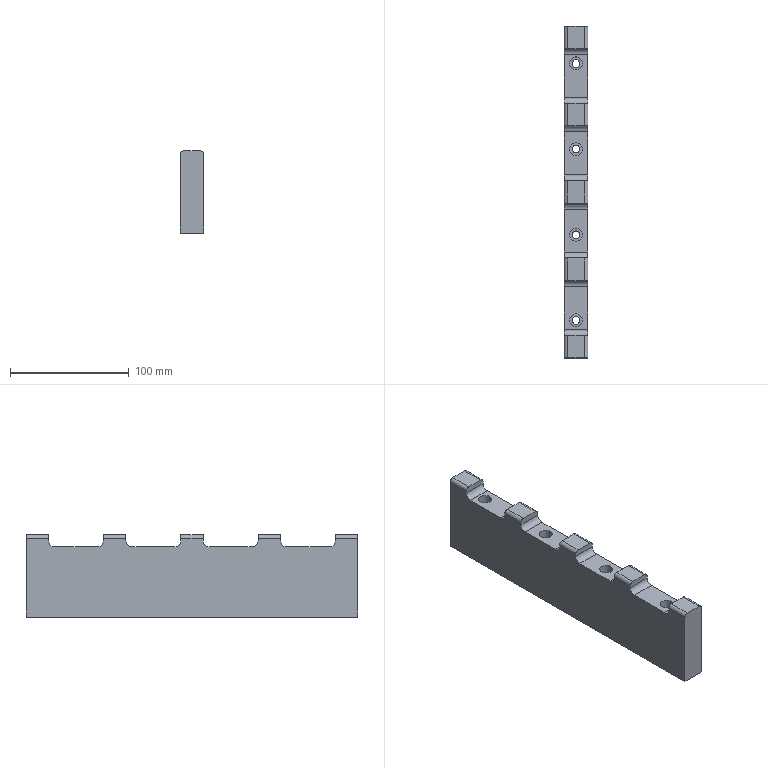Part | 1 solid | 52 faces | box 20 x 279 x 69 mm | volume 338406 mm3 | cylinder 26 | plane 26 | commonest cylinder face diameters 6 x10 10 x8 6.5 x4 11 x4